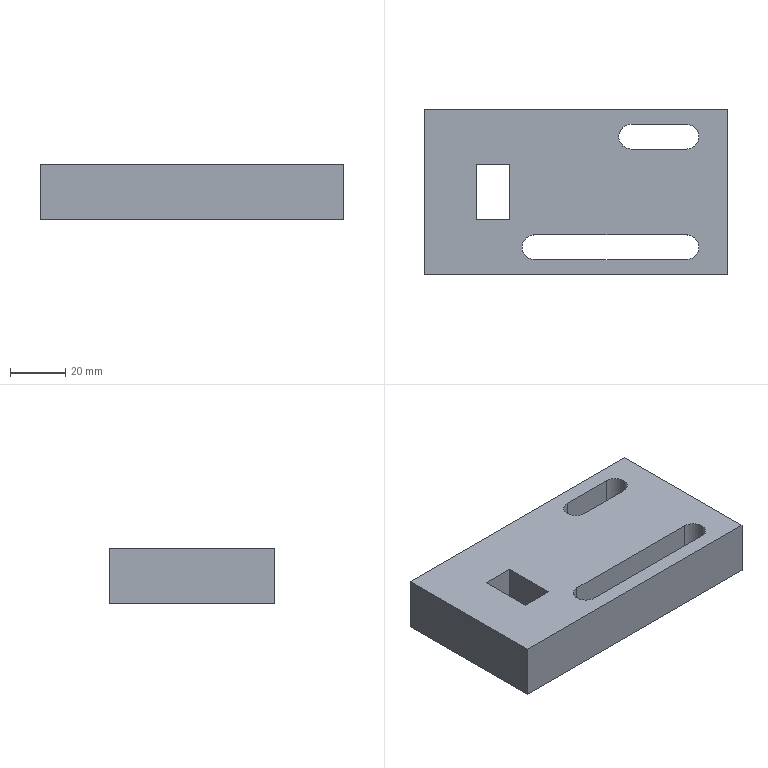Part | STEP file | 冲床-300配套压波_id190_x_t | 1 solid | 18 faces | box 110 x 60 x 20 mm | volume 111155 mm3 | plane 14 | cylinder 4 | commonest cylinder face diameters 9 x4
STEP:
#1=CARTESIAN_POINT('',(1145.,-209.5,20.));
#2=VERTEX_POINT('',#1);
#3=CARTESIAN_POINT('',(1145.,-200.5,20.));
#4=VERTEX_POINT('',#3);
#5=CARTESIAN_POINT('',(1145.,-205.,20.));
#6=DIRECTION('',(0.,0.,-1.));
#7=DIRECTION('',(1.,0.,0.));
#8=AXIS2_PLACEMENT_3D('',#5,#6,#7);
#9=CIRCLE('',#8,4.5);
#10=EDGE_CURVE('',#2,#4,#9,.T.);
#11=ORIENTED_EDGE('',*,*,#10,.F.);
#12=CARTESIAN_POINT('',(1145.,-209.5,0.));
#13=VERTEX_POINT('',#12);
#14=CARTESIAN_POINT('',(1145.,-209.5,0.));
#15=DIRECTION('',(0.,0.,-1.));
#16=VECTOR('',#15,1.);
#17=LINE('',#14,#16);
#18=EDGE_CURVE('',#2,#13,#17,.T.);
#19=ORIENTED_EDGE('',*,*,#18,.T.);
#20=CARTESIAN_POINT('',(1145.,-200.5,0.));
#21=VERTEX_POINT('',#20);
#22=CARTESIAN_POINT('',(1145.,-205.,0.));
#23=DIRECTION('',(0.,0.,-1.));
#24=DIRECTION('',(1.,0.,0.));
#25=AXIS2_PLACEMENT_3D('',#22,#23,#24);
#26=CIRCLE('',#25,4.5);
#27=EDGE_CURVE('',#13,#21,#26,.T.);
#28=ORIENTED_EDGE('',*,*,#27,.T.);
#29=CARTESIAN_POINT('',(1145.,-200.5,0.));
#30=DIRECTION('',(0.,0.,-1.));
#31=VECTOR('',#30,1.);
#32=LINE('',#29,#31);
#33=EDGE_CURVE('',#4,#21,#32,.T.);
#34=ORIENTED_EDGE('',*,*,#33,.F.);
#35=EDGE_LOOP('',(#11,#19,#28,#34));
#36=FACE_OUTER_BOUND('',#35,.T.);
#37=CARTESIAN_POINT('',(1145.,-205.,0.));
#38=DIRECTION('',(0.,0.,1.));
#39=DIRECTION('',(-1.,0.,0.));
#40=AXIS2_PLACEMENT_3D('',#37,#38,#39);
#41=CYLINDRICAL_SURFACE('',#40,4.5);
#42=ADVANCED_FACE('',(#36),#41,.F.);
#43=CARTESIAN_POINT('',(1180.,-160.5,20.));
#44=VERTEX_POINT('',#43);
#45=CARTESIAN_POINT('',(1200.,-160.5,20.));
#46=VERTEX_POINT('',#45);
#47=CARTESIAN_POINT('',(1200.,-160.5,20.));
#48=DIRECTION('',(1.,0.,0.));
#49=VECTOR('',#48,1.);
#50=LINE('',#47,#49);
#51=EDGE_CURVE('',#44,#46,#50,.T.);
#52=ORIENTED_EDGE('',*,*,#51,.F.);
#53=CARTESIAN_POINT('',(1180.,-160.5,0.));
#54=VERTEX_POINT('',#53);
#55=CARTESIAN_POINT('',(1180.,-160.5,0.));
#56=DIRECTION('',(0.,0.,1.));
#57=VECTOR('',#56,1.);
#58=LINE('',#55,#57);
#59=EDGE_CURVE('',#54,#44,#58,.T.);
#60=ORIENTED_EDGE('',*,*,#59,.F.);
#61=CARTESIAN_POINT('',(1200.,-160.5,0.));
#62=VERTEX_POINT('',#61);
#63=CARTESIAN_POINT('',(1200.,-160.5,0.));
#64=DIRECTION('',(1.,0.,0.));
#65=VECTOR('',#64,1.);
#66=LINE('',#63,#65);
#67=EDGE_CURVE('',#54,#62,#66,.T.);
#68=ORIENTED_EDGE('',*,*,#67,.T.);
#69=CARTESIAN_POINT('',(1200.,-160.5,0.));
#70=DIRECTION('',(0.,0.,1.));
#71=VECTOR('',#70,1.);
#72=LINE('',#69,#71);
#73=EDGE_CURVE('',#62,#46,#72,.T.);
#74=ORIENTED_EDGE('',*,*,#73,.T.);
#75=EDGE_LOOP('',(#52,#60,#68,#74));
#76=FACE_OUTER_BOUND('',#75,.T.);
#77=CARTESIAN_POINT('',(1200.,-160.5,0.));
#78=DIRECTION('',(0.,-1.,0.));
#79=DIRECTION('',(0.,0.,1.));
#80=AXIS2_PLACEMENT_3D('',#77,#78,#79);
#81=PLANE('',#80);
#82=ADVANCED_FACE('',(#76),#81,.T.);
#83=CARTESIAN_POINT('',(1200.,-169.5,20.));
#84=VERTEX_POINT('',#83);
#85=CARTESIAN_POINT('',(1200.,-165.,20.));
#86=DIRECTION('',(0.,0.,-1.));
#87=DIRECTION('',(-1.,0.,0.));
#88=AXIS2_PLACEMENT_3D('',#85,#86,#87);
#89=CIRCLE('',#88,4.5);
#90=EDGE_CURVE('',#46,#84,#89,.T.);
#91=ORIENTED_EDGE('',*,*,#90,.F.);
#92=ORIENTED_EDGE('',*,*,#73,.F.);
#93=CARTESIAN_POINT('',(1200.,-169.5,0.));
#94=VERTEX_POINT('',#93);
#95=CARTESIAN_POINT('',(1200.,-165.,0.));
#96=DIRECTION('',(0.,0.,-1.));
#97=DIRECTION('',(-1.,0.,0.));
#98=AXIS2_PLACEMENT_3D('',#95,#96,#97);
#99=CIRCLE('',#98,4.5);
#100=EDGE_CURVE('',#62,#94,#99,.T.);
#101=ORIENTED_EDGE('',*,*,#100,.T.);
#102=CARTESIAN_POINT('',(1200.,-169.5,0.));
#103=DIRECTION('',(0.,0.,1.));
#104=VECTOR('',#103,1.);
#105=LINE('',#102,#104);
#106=EDGE_CURVE('',#94,#84,#105,.T.);
#107=ORIENTED_EDGE('',*,*,#106,.T.);
#108=EDGE_LOOP('',(#91,#92,#101,#107));
#109=FACE_OUTER_BOUND('',#108,.T.);
#110=CARTESIAN_POINT('',(1200.,-165.,0.));
#111=DIRECTION('',(0.,0.,1.));
#112=DIRECTION('',(1.,0.,0.));
#113=AXIS2_PLACEMENT_3D('',#110,#111,#112);
#114=CYLINDRICAL_SURFACE('',#113,4.5);
#115=ADVANCED_FACE('',(#109),#114,.F.);
#116=CARTESIAN_POINT('',(1180.,-169.5,20.));
#117=VERTEX_POINT('',#116);
#118=CARTESIAN_POINT('',(1180.,-169.5,20.));
#119=DIRECTION('',(-1.,0.,0.));
#120=VECTOR('',#119,1.);
#121=LINE('',#118,#120);
#122=EDGE_CURVE('',#84,#117,#121,.T.);
#123=ORIENTED_EDGE('',*,*,#122,.F.);
#124=ORIENTED_EDGE('',*,*,#106,.F.);
#125=CARTESIAN_POINT('',(1180.,-169.5,0.));
#126=VERTEX_POINT('',#125);
#127=CARTESIAN_POINT('',(1180.,-169.5,0.));
#128=DIRECTION('',(-1.,0.,0.));
#129=VECTOR('',#128,1.);
#130=LINE('',#127,#129);
#131=EDGE_CURVE('',#94,#126,#130,.T.);
#132=ORIENTED_EDGE('',*,*,#131,.T.);
#133=CARTESIAN_POINT('',(1180.,-169.5,0.));
#134=DIRECTION('',(0.,0.,1.));
#135=VECTOR('',#134,1.);
#136=LINE('',#133,#135);
#137=EDGE_CURVE('',#126,#117,#136,.T.);
#138=ORIENTED_EDGE('',*,*,#137,.T.);
#139=EDGE_LOOP('',(#123,#124,#132,#138));
#140=FACE_OUTER_BOUND('',#139,.T.);
#141=CARTESIAN_POINT('',(1180.,-169.5,0.));
#142=DIRECTION('',(0.,1.,0.));
#143=DIRECTION('',(0.,0.,-1.));
#144=AXIS2_PLACEMENT_3D('',#141,#142,#143);
#145=PLANE('',#144);
#146=ADVANCED_FACE('',(#140),#145,.T.);
#147=CARTESIAN_POINT('',(1180.,-165.,20.));
#148=DIRECTION('',(0.,0.,-1.));
#149=DIRECTION('',(-1.,0.,0.));
#150=AXIS2_PLACEMENT_3D('',#147,#148,#149);
#151=CIRCLE('',#150,4.5);
#152=EDGE_CURVE('',#117,#44,#151,.T.);
#153=ORIENTED_EDGE('',*,*,#152,.F.);
#154=ORIENTED_EDGE('',*,*,#137,.F.);
#155=CARTESIAN_POINT('',(1180.,-165.,0.));
#156=DIRECTION('',(0.,0.,-1.));
#157=DIRECTION('',(-1.,0.,0.));
#158=AXIS2_PLACEMENT_3D('',#155,#156,#157);
#159=CIRCLE('',#158,4.5);
#160=EDGE_CURVE('',#126,#54,#159,.T.);
#161=ORIENTED_EDGE('',*,*,#160,.T.);
#162=ORIENTED_EDGE('',*,*,#59,.T.);
#163=EDGE_LOOP('',(#153,#154,#161,#162));
#164=FACE_OUTER_BOUND('',#163,.T.);
#165=CARTESIAN_POINT('',(1180.,-165.,0.));
#166=DIRECTION('',(0.,0.,1.));
#167=DIRECTION('',(1.,0.,0.));
#168=AXIS2_PLACEMENT_3D('',#165,#166,#167);
#169=CYLINDRICAL_SURFACE('',#168,4.5);
#170=ADVANCED_FACE('',(#164),#169,.F.);
#171=CARTESIAN_POINT('',(1200.,-200.5,20.));
#172=VERTEX_POINT('',#171);
#173=CARTESIAN_POINT('',(1200.,-209.5,20.));
#174=VERTEX_POINT('',#173);
#175=CARTESIAN_POINT('',(1200.,-205.,20.));
#176=DIRECTION('',(0.,0.,-1.));
#177=DIRECTION('',(-1.,0.,0.));
#178=AXIS2_PLACEMENT_3D('',#175,#176,#177);
#179=CIRCLE('',#178,4.5);
#180=EDGE_CURVE('',#172,#174,#179,.T.);
#181=ORIENTED_EDGE('',*,*,#180,.F.);
#182=CARTESIAN_POINT('',(1200.,-200.5,0.));
#183=VERTEX_POINT('',#182);
#184=CARTESIAN_POINT('',(1200.,-200.5,0.));
#185=DIRECTION('',(0.,0.,1.));
#186=VECTOR('',#185,1.);
#187=LINE('',#184,#186);
#188=EDGE_CURVE('',#183,#172,#187,.T.);
#189=ORIENTED_EDGE('',*,*,#188,.F.);
#190=CARTESIAN_POINT('',(1200.,-209.5,0.));
#191=VERTEX_POINT('',#190);
#192=CARTESIAN_POINT('',(1200.,-205.,0.));
#193=DIRECTION('',(0.,0.,-1.));
#194=DIRECTION('',(-1.,0.,0.));
#195=AXIS2_PLACEMENT_3D('',#192,#193,#194);
#196=CIRCLE('',#195,4.5);
#197=EDGE_CURVE('',#183,#191,#196,.T.);
#198=ORIENTED_EDGE('',*,*,#197,.T.);
#199=CARTESIAN_POINT('',(1200.,-209.5,0.));
#200=DIRECTION('',(0.,0.,1.));
#201=VECTOR('',#200,1.);
#202=LINE('',#199,#201);
#203=EDGE_CURVE('',#191,#174,#202,.T.);
#204=ORIENTED_EDGE('',*,*,#203,.T.);
#205=EDGE_LOOP('',(#181,#189,#198,#204));
#206=FACE_OUTER_BOUND('',#205,.T.);
#207=CARTESIAN_POINT('',(1200.,-205.,0.));
#208=DIRECTION('',(0.,0.,1.));
#209=DIRECTION('',(1.,0.,0.));
#210=AXIS2_PLACEMENT_3D('',#207,#208,#209);
#211=CYLINDRICAL_SURFACE('',#210,4.5);
#212=ADVANCED_FACE('',(#206),#211,.F.);
#213=CARTESIAN_POINT('',(1180.,-209.5,20.));
#214=DIRECTION('',(-1.,0.,0.));
#215=VECTOR('',#214,1.);
#216=LINE('',#213,#215);
#217=EDGE_CURVE('',#174,#2,#216,.T.);
#218=ORIENTED_EDGE('',*,*,#217,.F.);
#219=ORIENTED_EDGE('',*,*,#203,.F.);
#220=CARTESIAN_POINT('',(1180.,-209.5,0.));
#221=DIRECTION('',(-1.,0.,0.));
#222=VECTOR('',#221,1.);
#223=LINE('',#220,#222);
#224=EDGE_CURVE('',#191,#13,#223,.T.);
#225=ORIENTED_EDGE('',*,*,#224,.T.);
#226=ORIENTED_EDGE('',*,*,#18,.F.);
#227=EDGE_LOOP('',(#218,#219,#225,#226));
#228=FACE_OUTER_BOUND('',#227,.T.);
#229=CARTESIAN_POINT('',(1180.,-209.5,0.));
#230=DIRECTION('',(0.,1.,0.));
#231=DIRECTION('',(0.,0.,-1.));
#232=AXIS2_PLACEMENT_3D('',#229,#230,#231);
#233=PLANE('',#232);
#234=ADVANCED_FACE('',(#228),#233,.T.);
#235=CARTESIAN_POINT('',(1200.,-200.5,20.));
#236=DIRECTION('',(1.,0.,0.));
#237=VECTOR('',#236,1.);
#238=LINE('',#235,#237);
#239=EDGE_CURVE('',#4,#172,#238,.T.);
#240=ORIENTED_EDGE('',*,*,#239,.F.);
#241=ORIENTED_EDGE('',*,*,#33,.T.);
#242=CARTESIAN_POINT('',(1200.,-200.5,0.));
#243=DIRECTION('',(1.,0.,0.));
#244=VECTOR('',#243,1.);
#245=LINE('',#242,#244);
#246=EDGE_CURVE('',#21,#183,#245,.T.);
#247=ORIENTED_EDGE('',*,*,#246,.T.);
#248=ORIENTED_EDGE('',*,*,#188,.T.);
#249=EDGE_LOOP('',(#240,#241,#247,#248));
#250=FACE_OUTER_BOUND('',#249,.T.);
#251=CARTESIAN_POINT('',(1200.,-200.5,0.));
#252=DIRECTION('',(0.,-1.,0.));
#253=DIRECTION('',(0.,0.,1.));
#254=AXIS2_PLACEMENT_3D('',#251,#252,#253);
#255=PLANE('',#254);
#256=ADVANCED_FACE('',(#250),#255,.T.);
#257=CARTESIAN_POINT('',(1215.,-215.,20.));
#258=VERTEX_POINT('',#257);
#259=CARTESIAN_POINT('',(1215.,-155.,20.));
#260=VERTEX_POINT('',#259);
#261=CARTESIAN_POINT('',(1215.,-195.,20.));
#262=DIRECTION('',(0.,1.,0.));
#263=VECTOR('',#262,1.);
#264=LINE('',#261,#263);
#265=EDGE_CURVE('',#258,#260,#264,.T.);
#266=ORIENTED_EDGE('',*,*,#265,.F.);
#267=CARTESIAN_POINT('',(1215.,-215.,0.));
#268=VERTEX_POINT('',#267);
#269=CARTESIAN_POINT('',(1215.,-215.,0.));
#270=DIRECTION('',(0.,0.,-1.));
#271=VECTOR('',#270,1.);
#272=LINE('',#269,#271);
#273=EDGE_CURVE('',#258,#268,#272,.T.);
#274=ORIENTED_EDGE('',*,*,#273,.T.);
#275=CARTESIAN_POINT('',(1215.,-155.,0.));
#276=VERTEX_POINT('',#275);
#277=CARTESIAN_POINT('',(1215.,-195.,0.));
#278=DIRECTION('',(0.,1.,0.));
#279=VECTOR('',#278,1.);
#280=LINE('',#277,#279);
#281=EDGE_CURVE('',#268,#276,#280,.T.);
#282=ORIENTED_EDGE('',*,*,#281,.T.);
#283=CARTESIAN_POINT('',(1215.,-155.,0.));
#284=DIRECTION('',(0.,0.,1.));
#285=VECTOR('',#284,1.);
#286=LINE('',#283,#285);
#287=EDGE_CURVE('',#276,#260,#286,.T.);
#288=ORIENTED_EDGE('',*,*,#287,.T.);
#289=EDGE_LOOP('',(#266,#274,#282,#288));
#290=FACE_OUTER_BOUND('',#289,.T.);
#291=CARTESIAN_POINT('',(1215.,-195.,0.));
#292=DIRECTION('',(1.,0.,0.));
#293=DIRECTION('',(0.,-1.,0.));
#294=AXIS2_PLACEMENT_3D('',#291,#292,#293);
#295=PLANE('',#294);
#296=ADVANCED_FACE('',(#290),#295,.T.);
#297=ORIENTED_EDGE('',*,*,#287,.F.);
#298=CARTESIAN_POINT('',(1105.,-155.,0.));
#299=VERTEX_POINT('',#298);
#300=CARTESIAN_POINT('',(1105.,-155.,0.));
#301=DIRECTION('',(1.,0.,0.));
#302=VECTOR('',#301,1.);
#303=LINE('',#300,#302);
#304=EDGE_CURVE('',#299,#276,#303,.T.);
#305=ORIENTED_EDGE('',*,*,#304,.F.);
#306=CARTESIAN_POINT('',(1105.,-155.,20.));
#307=VERTEX_POINT('',#306);
#308=CARTESIAN_POINT('',(1105.,-155.,0.));
#309=DIRECTION('',(0.,0.,1.));
#310=VECTOR('',#309,1.);
#311=LINE('',#308,#310);
#312=EDGE_CURVE('',#299,#307,#311,.T.);
#313=ORIENTED_EDGE('',*,*,#312,.T.);
#314=CARTESIAN_POINT('',(1105.,-155.,20.));
#315=DIRECTION('',(1.,0.,0.));
#316=VECTOR('',#315,1.);
#317=LINE('',#314,#316);
#318=EDGE_CURVE('',#307,#260,#317,.T.);
#319=ORIENTED_EDGE('',*,*,#318,.T.);
#320=EDGE_LOOP('',(#297,#305,#313,#319));
#321=FACE_OUTER_BOUND('',#320,.T.);
#322=CARTESIAN_POINT('',(1105.,-155.,0.));
#323=DIRECTION('',(0.,-1.,0.));
#324=DIRECTION('',(1.,0.,0.));
#325=AXIS2_PLACEMENT_3D('',#322,#323,#324);
#326=PLANE('',#325);
#327=ADVANCED_FACE('',(#321),#326,.F.);
#328=CARTESIAN_POINT('',(1105.,-215.,0.));
#329=VERTEX_POINT('',#328);
#330=CARTESIAN_POINT('',(1105.,-195.,0.));
#331=DIRECTION('',(0.,1.,0.));
#332=VECTOR('',#331,1.);
#333=LINE('',#330,#332);
#334=EDGE_CURVE('',#329,#299,#333,.T.);
#335=ORIENTED_EDGE('',*,*,#334,.F.);
#336=CARTESIAN_POINT('',(1105.,-215.,20.));
#337=VERTEX_POINT('',#336);
#338=CARTESIAN_POINT('',(1105.,-215.,0.));
#339=DIRECTION('',(0.,0.,-1.));
#340=VECTOR('',#339,1.);
#341=LINE('',#338,#340);
#342=EDGE_CURVE('',#337,#329,#341,.T.);
#343=ORIENTED_EDGE('',*,*,#342,.F.);
#344=CARTESIAN_POINT('',(1105.,-195.,20.));
#345=DIRECTION('',(0.,1.,0.));
#346=VECTOR('',#345,1.);
#347=LINE('',#344,#346);
#348=EDGE_CURVE('',#337,#307,#347,.T.);
#349=ORIENTED_EDGE('',*,*,#348,.T.);
#350=ORIENTED_EDGE('',*,*,#312,.F.);
#351=EDGE_LOOP('',(#335,#343,#349,#350));
#352=FACE_OUTER_BOUND('',#351,.T.);
#353=CARTESIAN_POINT('',(1105.,-195.,0.));
#354=DIRECTION('',(1.,0.,0.));
#355=DIRECTION('',(0.,-1.,0.));
#356=AXIS2_PLACEMENT_3D('',#353,#354,#355);
#357=PLANE('',#356);
#358=ADVANCED_FACE('',(#352),#357,.F.);
#359=ORIENTED_EDGE('',*,*,#273,.F.);
#360=CARTESIAN_POINT('',(1105.,-215.,20.));
#361=DIRECTION('',(-1.,0.,0.));
#362=VECTOR('',#361,1.);
#363=LINE('',#360,#362);
#364=EDGE_CURVE('',#258,#337,#363,.T.);
#365=ORIENTED_EDGE('',*,*,#364,.T.);
#366=ORIENTED_EDGE('',*,*,#342,.T.);
#367=CARTESIAN_POINT('',(1105.,-215.,0.));
#368=DIRECTION('',(-1.,0.,0.));
#369=VECTOR('',#368,1.);
#370=LINE('',#367,#369);
#371=EDGE_CURVE('',#268,#329,#370,.T.);
#372=ORIENTED_EDGE('',*,*,#371,.F.);
#373=EDGE_LOOP('',(#359,#365,#366,#372));
#374=FACE_OUTER_BOUND('',#373,.T.);
#375=CARTESIAN_POINT('',(1105.,-215.,0.));
#376=DIRECTION('',(0.,1.,0.));
#377=DIRECTION('',(1.,0.,0.));
#378=AXIS2_PLACEMENT_3D('',#375,#376,#377);
#379=PLANE('',#378);
#380=ADVANCED_FACE('',(#374),#379,.F.);
#381=CARTESIAN_POINT('',(1136.,-175.,20.));
#382=VERTEX_POINT('',#381);
#383=CARTESIAN_POINT('',(1124.,-175.,20.));
#384=VERTEX_POINT('',#383);
#385=CARTESIAN_POINT('',(1105.,-175.,20.));
#386=DIRECTION('',(-1.,0.,0.));
#387=VECTOR('',#386,1.);
#388=LINE('',#385,#387);
#389=EDGE_CURVE('',#382,#384,#388,.T.);
#390=ORIENTED_EDGE('',*,*,#389,.T.);
#391=CARTESIAN_POINT('',(1124.,-175.,0.));
#392=VERTEX_POINT('',#391);
#393=CARTESIAN_POINT('',(1124.,-175.,20.));
#394=DIRECTION('',(0.,0.,-1.));
#395=VECTOR('',#394,1.);
#396=LINE('',#393,#395);
#397=EDGE_CURVE('',#384,#392,#396,.T.);
#398=ORIENTED_EDGE('',*,*,#397,.T.);
#399=CARTESIAN_POINT('',(1136.,-175.,0.));
#400=VERTEX_POINT('',#399);
#401=CARTESIAN_POINT('',(1124.,-175.,0.));
#402=DIRECTION('',(-1.,0.,0.));
#403=VECTOR('',#402,1.);
#404=LINE('',#401,#403);
#405=EDGE_CURVE('',#400,#392,#404,.T.);
#406=ORIENTED_EDGE('',*,*,#405,.F.);
#407=CARTESIAN_POINT('',(1136.,-175.,0.));
#408=DIRECTION('',(0.,0.,1.));
#409=VECTOR('',#408,1.);
#410=LINE('',#407,#409);
#411=EDGE_CURVE('',#400,#382,#410,.T.);
#412=ORIENTED_EDGE('',*,*,#411,.T.);
#413=EDGE_LOOP('',(#390,#398,#406,#412));
#414=FACE_OUTER_BOUND('',#413,.T.);
#415=CARTESIAN_POINT('',(1155.,-175.,50.));
#416=DIRECTION('',(0.,1.,0.));
#417=DIRECTION('',(0.,0.,-1.));
#418=AXIS2_PLACEMENT_3D('',#415,#416,#417);
#419=PLANE('',#418);
#420=ADVANCED_FACE('',(#414),#419,.F.);
#421=CARTESIAN_POINT('',(1136.,-195.,0.));
#422=VERTEX_POINT('',#421);
#423=CARTESIAN_POINT('',(1136.,-195.,20.));
#424=VERTEX_POINT('',#423);
#425=CARTESIAN_POINT('',(1136.,-195.,0.));
#426=DIRECTION('',(0.,0.,1.));
#427=VECTOR('',#426,1.);
#428=LINE('',#425,#427);
#429=EDGE_CURVE('',#422,#424,#428,.T.);
#430=ORIENTED_EDGE('',*,*,#429,.T.);
#431=CARTESIAN_POINT('',(1136.,-175.,20.));
#432=DIRECTION('',(0.,1.,0.));
#433=VECTOR('',#432,1.);
#434=LINE('',#431,#433);
#435=EDGE_CURVE('',#424,#382,#434,.T.);
#436=ORIENTED_EDGE('',*,*,#435,.T.);
#437=ORIENTED_EDGE('',*,*,#411,.F.);
#438=CARTESIAN_POINT('',(1136.,-175.,0.));
#439=DIRECTION('',(0.,-1.,0.));
#440=VECTOR('',#439,1.);
#441=LINE('',#438,#440);
#442=EDGE_CURVE('',#400,#422,#441,.T.);
#443=ORIENTED_EDGE('',*,*,#442,.T.);
#444=EDGE_LOOP('',(#430,#436,#437,#443));
#445=FACE_OUTER_BOUND('',#444,.T.);
#446=CARTESIAN_POINT('',(1136.,-175.,0.));
#447=DIRECTION('',(1.,0.,0.));
#448=DIRECTION('',(0.,0.,1.));
#449=AXIS2_PLACEMENT_3D('',#446,#447,#448);
#450=PLANE('',#449);
#451=ADVANCED_FACE('',(#445),#450,.F.);
#452=CARTESIAN_POINT('',(1124.,-195.,20.));
#453=VERTEX_POINT('',#452);
#454=CARTESIAN_POINT('',(1124.,-195.,0.));
#455=VERTEX_POINT('',#454);
#456=CARTESIAN_POINT('',(1124.,-195.,20.));
#457=DIRECTION('',(0.,0.,-1.));
#458=VECTOR('',#457,1.);
#459=LINE('',#456,#458);
#460=EDGE_CURVE('',#453,#455,#459,.T.);
#461=ORIENTED_EDGE('',*,*,#460,.F.);
#462=CARTESIAN_POINT('',(1105.,-195.,20.));
#463=DIRECTION('',(-1.,0.,0.));
#464=VECTOR('',#463,1.);
#465=LINE('',#462,#464);
#466=EDGE_CURVE('',#424,#453,#465,.T.);
#467=ORIENTED_EDGE('',*,*,#466,.F.);
#468=ORIENTED_EDGE('',*,*,#429,.F.);
#469=CARTESIAN_POINT('',(1124.,-195.,0.));
#470=DIRECTION('',(-1.,0.,0.));
#471=VECTOR('',#470,1.);
#472=LINE('',#469,#471);
#473=EDGE_CURVE('',#422,#455,#472,.T.);
#474=ORIENTED_EDGE('',*,*,#473,.T.);
#475=EDGE_LOOP('',(#461,#467,#468,#474));
#476=FACE_OUTER_BOUND('',#475,.T.);
#477=CARTESIAN_POINT('',(1155.,-195.,50.));
#478=DIRECTION('',(0.,1.,0.));
#479=DIRECTION('',(0.,0.,-1.));
#480=AXIS2_PLACEMENT_3D('',#477,#478,#479);
#481=PLANE('',#480);
#482=ADVANCED_FACE('',(#476),#481,.T.);
#483=ORIENTED_EDGE('',*,*,#460,.T.);
#484=CARTESIAN_POINT('',(1124.,-175.,0.));
#485=DIRECTION('',(0.,-1.,0.));
#486=VECTOR('',#485,1.);
#487=LINE('',#484,#486);
#488=EDGE_CURVE('',#392,#455,#487,.T.);
#489=ORIENTED_EDGE('',*,*,#488,.F.);
#490=ORIENTED_EDGE('',*,*,#397,.F.);
#491=CARTESIAN_POINT('',(1124.,-175.,20.));
#492=DIRECTION('',(0.,-1.,0.));
#493=VECTOR('',#492,1.);
#494=LINE('',#491,#493);
#495=EDGE_CURVE('',#384,#453,#494,.T.);
#496=ORIENTED_EDGE('',*,*,#495,.T.);
#497=EDGE_LOOP('',(#483,#489,#490,#496));
#498=FACE_OUTER_BOUND('',#497,.T.);
#499=CARTESIAN_POINT('',(1124.,-175.,20.));
#500=DIRECTION('',(-1.,0.,0.));
#501=DIRECTION('',(0.,0.,-1.));
#502=AXIS2_PLACEMENT_3D('',#499,#500,#501);
#503=PLANE('',#502);
#504=ADVANCED_FACE('',(#498),#503,.F.);
#505=ORIENTED_EDGE('',*,*,#239,.T.);
#506=ORIENTED_EDGE('',*,*,#180,.T.);
#507=ORIENTED_EDGE('',*,*,#217,.T.);
#508=ORIENTED_EDGE('',*,*,#10,.T.);
#509=EDGE_LOOP('',(#505,#506,#507,#508));
#510=FACE_BOUND('',#509,.T.);
#511=ORIENTED_EDGE('',*,*,#495,.F.);
#512=ORIENTED_EDGE('',*,*,#389,.F.);
#513=ORIENTED_EDGE('',*,*,#435,.F.);
#514=ORIENTED_EDGE('',*,*,#466,.T.);
#515=EDGE_LOOP('',(#511,#512,#513,#514));
#516=FACE_BOUND('',#515,.T.);
#517=ORIENTED_EDGE('',*,*,#364,.F.);
#518=ORIENTED_EDGE('',*,*,#265,.T.);
#519=ORIENTED_EDGE('',*,*,#318,.F.);
#520=ORIENTED_EDGE('',*,*,#348,.F.);
#521=EDGE_LOOP('',(#517,#518,#519,#520));
#522=FACE_BOUND('',#521,.T.);
#523=ORIENTED_EDGE('',*,*,#152,.T.);
#524=ORIENTED_EDGE('',*,*,#51,.T.);
#525=ORIENTED_EDGE('',*,*,#90,.T.);
#526=ORIENTED_EDGE('',*,*,#122,.T.);
#527=EDGE_LOOP('',(#523,#524,#525,#526));
#528=FACE_BOUND('',#527,.T.);
#529=CARTESIAN_POINT('',(1105.,-195.,20.));
#530=DIRECTION('',(0.,0.,1.));
#531=DIRECTION('',(1.,0.,0.));
#532=AXIS2_PLACEMENT_3D('',#529,#530,#531);
#533=PLANE('',#532);
#534=ADVANCED_FACE('',(#510,#516,#522,#528),#533,.T.);
#535=ORIENTED_EDGE('',*,*,#27,.F.);
#536=ORIENTED_EDGE('',*,*,#224,.F.);
#537=ORIENTED_EDGE('',*,*,#197,.F.);
#538=ORIENTED_EDGE('',*,*,#246,.F.);
#539=EDGE_LOOP('',(#535,#536,#537,#538));
#540=FACE_BOUND('',#539,.T.);
#541=ORIENTED_EDGE('',*,*,#371,.T.);
#542=ORIENTED_EDGE('',*,*,#334,.T.);
#543=ORIENTED_EDGE('',*,*,#304,.T.);
#544=ORIENTED_EDGE('',*,*,#281,.F.);
#545=EDGE_LOOP('',(#541,#542,#543,#544));
#546=FACE_BOUND('',#545,.T.);
#547=ORIENTED_EDGE('',*,*,#442,.F.);
#548=ORIENTED_EDGE('',*,*,#405,.T.);
#549=ORIENTED_EDGE('',*,*,#488,.T.);
#550=ORIENTED_EDGE('',*,*,#473,.F.);
#551=EDGE_LOOP('',(#547,#548,#549,#550));
#552=FACE_BOUND('',#551,.T.);
#553=ORIENTED_EDGE('',*,*,#131,.F.);
#554=ORIENTED_EDGE('',*,*,#100,.F.);
#555=ORIENTED_EDGE('',*,*,#67,.F.);
#556=ORIENTED_EDGE('',*,*,#160,.F.);
#557=EDGE_LOOP('',(#553,#554,#555,#556));
#558=FACE_BOUND('',#557,.T.);
#559=CARTESIAN_POINT('',(1105.,-195.,0.));
#560=DIRECTION('',(0.,0.,1.));
#561=DIRECTION('',(1.,0.,0.));
#562=AXIS2_PLACEMENT_3D('',#559,#560,#561);
#563=PLANE('',#562);
#564=ADVANCED_FACE('',(#540,#546,#552,#558),#563,.F.);
#565=CLOSED_SHELL('',(#42,#82,#115,#146,#170,#212,#234,#256,#296,#327,#358,#380,#420,#451,#482,#504,#534,#564));
#566=MANIFOLD_SOLID_BREP('',#565);
#567=(LENGTH_UNIT()NAMED_UNIT(*)SI_UNIT(.MILLI.,.METRE.));
#568=UNCERTAINTY_MEASURE_WITH_UNIT(LENGTH_MEASURE(0.00002),#567,'','');
#569=(NAMED_UNIT(*)PLANE_ANGLE_UNIT()SI_UNIT($,.RADIAN.));
#570=PLANE_ANGLE_MEASURE_WITH_UNIT(PLANE_ANGLE_MEASURE(0.01745),#569);
#571=DIMENSIONAL_EXPONENTS(0.,0.,0.,0.,0.,0.,0.);
#572=(CONVERSION_BASED_UNIT('DEGREE',#570)NAMED_UNIT(#571)PLANE_ANGLE_UNIT());
#573=(NAMED_UNIT(*)SI_UNIT($,.STERADIAN.)SOLID_ANGLE_UNIT());
#574=(GEOMETRIC_REPRESENTATION_CONTEXT(3)GLOBAL_UNCERTAINTY_ASSIGNED_CONTEXT((#568))GLOBAL_UNIT_ASSIGNED_CONTEXT((#567,#572,#573))REPRESENTATION_CONTEXT('',''));
#575=ADVANCED_BREP_SHAPE_REPRESENTATION('',(#566),#574);